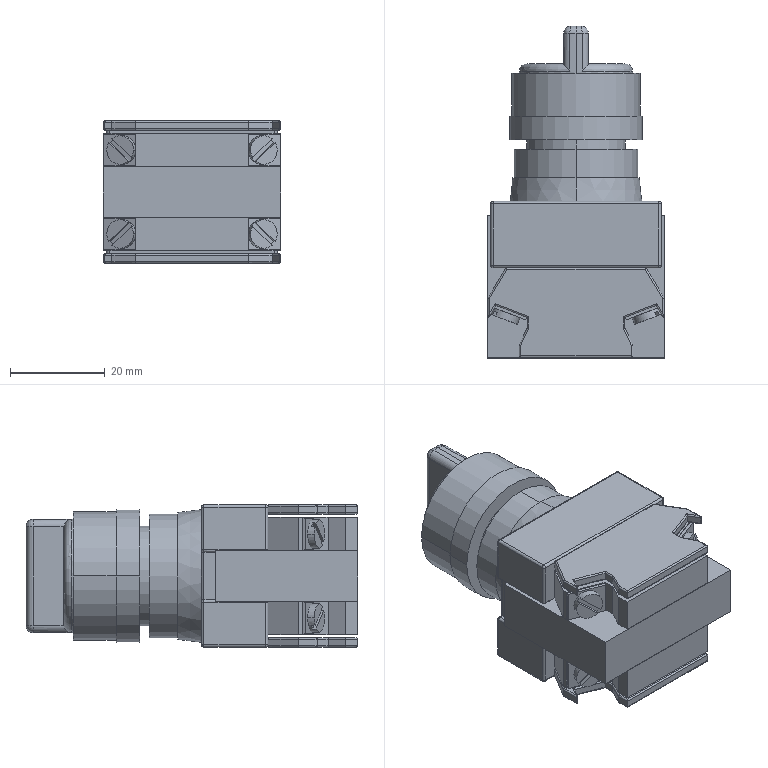Part | SolidWorks | features BaseBody 3, Fillet 2, ICE 2 | 3 solids | 297 faces | box 37.364 x 70 x 30 mm | volume 49458 mm3 | plane 136 | cylinder 126 | spline 24 | torus 5 | sphere 4 | cone 2 | commonest cylinder face diameters 0.6 x64 1 x34 6 x8 3 x6 0.24 x4 21 x2